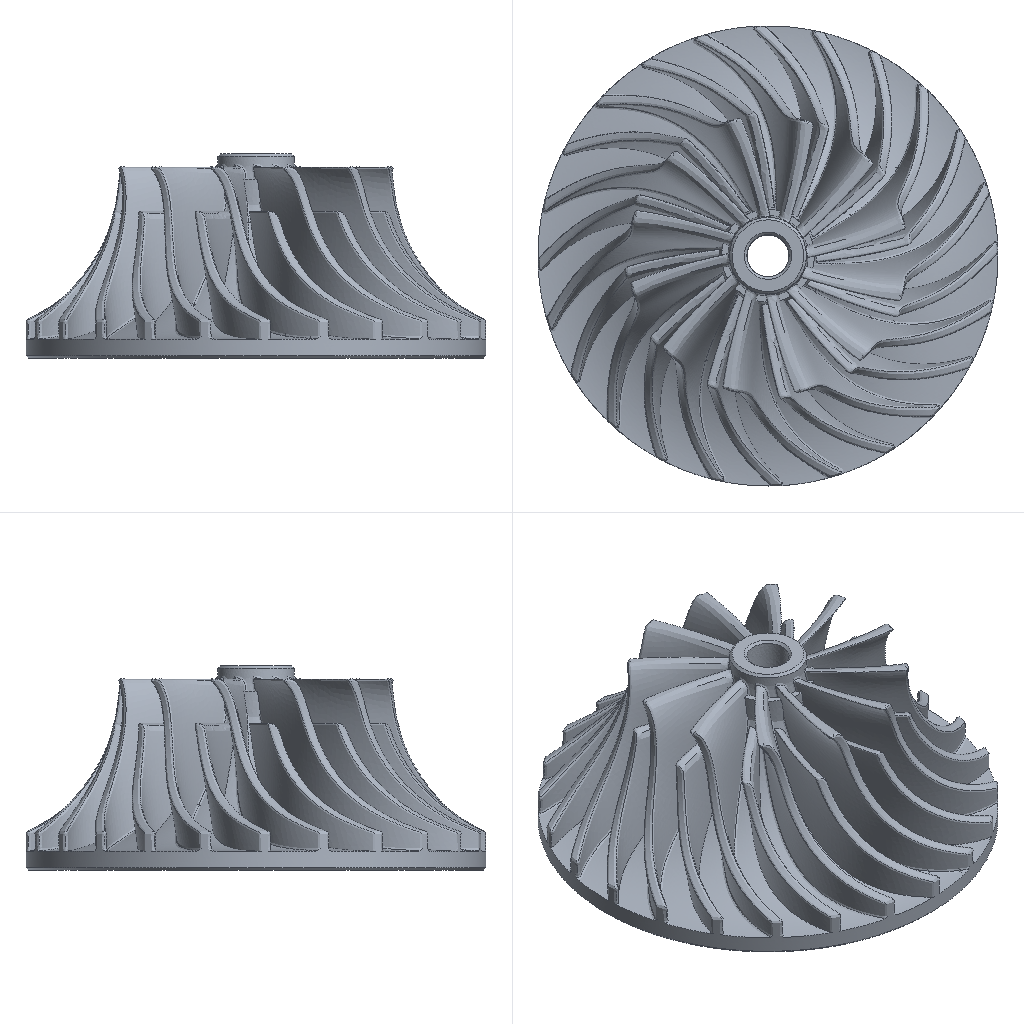Simulation study
Set-up summary:
category,name,step,type,value,unit,region
solver,ansys_mapdl
solver,version,,,22.2
units,MPA,,stated
analysis,deck,,static,static
load_step,requested,,,1
analysis,nlgeom,,,False
mesh,nodes,,,702794
mesh,elements,,,409743
element_type,ANSYS 187 (type 1),,solid,409743
load,load commands in deck,,count,1
bc,support commands in deck,,count,3
named_set,_DISPZEROUX,,component
named_set,_DISPZEROUY,,component
named_set,_DISPZEROUZ,,component
material,1,,in results
check,setup vs results,,match
Ansys APDL input file, long lists of numbers shortened:
/batch
/config,noeldb,1     ! force off writing results to database
*get,_wallstrt,active,,time,wall
! ANSYS input file written by Workbench version 2022 R2
! File used for geometry attach: D:\虚拟C盘\有限元\Impeller_v2.stp
/title,wbnew--____ (A5)
! ****** Begin Custom Load Command Snippet ******
/COM, ACT Extensions:
/COM,     LSDYNA, 2022.2
/COM,/COM,     ANSYSMotion, 2022.2
/COM,
! ****** End   Custom Load Command Snippet ******
*DIM,_wb_ProjectScratch_dir,string,248
_wb_ProjectScratch_dir(1) = 'C:\Users\16969\AppData\Local\Temp\WB_16969_1848_2\_ProjectScratch\ScrAECD\'
*DIM,_wb_SolverFiles_dir,string,248
_wb_SolverFiles_dir(1) = 'C:\Users\16969\AppData\Local\Temp\WB_16969_1848_2\wbnew_files\dp0\SYS\MECH\'
*DIM,_wb_userfiles_dir,string,248
_wb_userfiles_dir(1) = 'C:\Users\16969\AppData\Local\Temp\WB_16969_1848_2\wbnew_files\user_files\'
/com,--- Data in consistent NMM units. See Solving Units in the help system for more information.
/units,MPA
/nopr
/wb,file,start              !  signify a WB generated input file
/prep7
! Turn off shape checking because checks already performed inside WB mesher.
! See help system for more information.
SHPP,OFF,,NOWARN
/nolist
etcon,set             ! allow ANSYS to choose best KEYOP's for 180x elements, resets any applicable keyopt to MAPDL defaults
/com,*********** Nodes for the whole assembly ***********
nblock,3,,773073
(1i9,3e20.9e3)
        1    -1.739180704E+02     4.639509446E+01     1.500000000E+01
! (702793 more lines like these left out)
-1
/wb,elem,start            !  set before creation of elements
/com,*********** Elements for Body 1 "Impeller_v2-FreeParts|Impeller_v2" ***********
et,1,187
eblock,19,solid,,409743
(19i9)
        1        1        1        1        0        0        0        0       10        0        1    78715   108325    93396   101043   578094   670925   578088   578092
! (819485 more lines like these left out)
-1
/wb,elem,end               !  done creating elements
/com,*********** Send User Defined Coordinate System(s) ***********
csys,0
toffst,273.15,  ! Temperature offset from absolute zero
/com,*********** Set Reference Temperature ***********
tref,22.
/wb,mat,start              !  starting to send materials
/com,*********** Send Materials ***********
Temperature = 'TEMP' ! Temperature
MP,DENS,1,2.77e-09,	! tonne mm^-3
MP,ALPX,1,2.3e-05,	! C^-1
MP,C,1,875000000,	! mm^2 s^-2 C^-1
MPTEMP,,,,,,,,
MPTEMP,1,-100
MPTEMP,2,0
MPTEMP,3,100
MPTEMP,4,200
MPDATA,KXX,1, ,114,144,165,175,	! tonne mm s^-3 C^-1
MPTEMP,,,,,,,,
MPTEMP,,,,,,,,
MPTEMP,1,0
MPTEMP,2,20
MPTEMP,3,100
MPDATA,RSVX,1, ,2.43e-05,2.67e-05,3.63e-05,	! ohm mm
MPTEMP,,,,,,,,
MP,EX,1,75000,	! tonne s^-2 mm^-1
MP,NUXY,1,0.25,
MP,MURX,1,1,
/wb,mat,end                !  done sending materials
!************************* Model Summary ********************
!Impeller_v2-FreeParts|Impeller_v2,	铝合金,	matid,	1
!************************* End Model Summary ********************
! get the diagonal of the bounding box. Needed later for other things
*get,_xmin,node,,mnloc,x
*get,_ymin,node,,mnloc,y
*get,_zmin,node,,mnloc,z
*get,_xmax,node,,mxloc,x
*get,_ymax,node,,mxloc,y
*get,_zmax,node,,mxloc,z
_ASMDIAG=(_xmax-_xmin)*(_xmax-_xmin)+(_ymax-_ymin)*(_ymax-_ymin)+(_zmax-_zmin)*(_zmax-_zmin)
_ASMDIAG=SQRT(_ASMDIAG)
/wb,contact,start          !  starting to send contact
/wb,contact,end            !  done creating contacts
/golist
/wb,load,start             !  starting to send loads
/com,******* Constant Zero Displacement X *******
CMBLOCK,_DISPZEROUX,NODE,    11096
(8i10)
     19529     19530     19531     19532     19533     19534     19535     19536
! (1386 more lines like these left out)
cmsel,s,_DISPZEROUX
d,all,ux,0
nsel,all
/com,******* Constant Zero Displacement Y *******
CMBLOCK,_DISPZEROUY,NODE,    11096
(8i10)
     19529     19530     19531     19532     19533     19534     19535     19536
! (1386 more lines like these left out)
cmsel,s,_DISPZEROUY
d,all,uy,0
nsel,all
/com,******* Constant Zero Displacement Z *******
CMBLOCK,_DISPZEROUZ,NODE,    11096
(8i10)
     19529     19530     19531     19532     19533     19534     19535     19536
! (1386 more lines like these left out)
cmsel,s,_DISPZEROUZ
d,all,uz,0
nsel,all
/com,*********** Define Rotational Velocity ***********
cglo,0.,0.,80.
/gst,on,on
fini
*get,_numnode,node,0,count
*get,_numelem,elem,0,count
*get, _MAXELEMNUM, elem, 0, NUM, MAX
*get, _MAXNODENUM, node, 0, NUM, MAX
*get, _MAXELEMTYPE, etyp, 0, NUM, MAX
*get, _MAXREALCONST, rcon, 0, NUM, MAX
/go
/wb,load,end               !  done creating loads
/com,--- Number of total nodes = %_numnode%
/com,--- Number of contact elements = 0
/com,--- Number of spring elements = 0
/com,--- Number of bearing elements = 0
/com,--- Number of solid elements = 409743
/com,--- Number of condensed parts = 0
/com,--- Number of total elements = %_numelem%
*get,_wallbsol,active,,time,wall
/com,****************************************************************************
/com,*************************    SOLUTION       ********************************
/com,****************************************************************************
/solu
antype,0                   ! static analysis
_thickRatio=  1     ! Ratio of thick parts in the model
eqsl,pcg,1e-8,,,,,,1
cntr,print,1               ! print out contact info and also make no initial contact an error
dmpoption,emat,no             ! Don't combine emat file for DANSYS
dmpoption,esav,no             ! Don't combine esav file for DANSYS
nldiag,cont,iter           ! print out contact info each equilibrium iteration
rescontrol,,none                 ! Do not keep any restart files
/com,****************************************************
/com,******************* SOLVE FOR LS 1 OF 1 ****************
cgom,0.,0.,200.
/nopr
/gopr
nsub,1,1,1
time,1.
outres,erase
outres,all,none
outres,nsol,all,
outres,rsol,all
outres,eangl,all
outres,etmp,all
outres,veng,all
outres,strs,all,
outres,epel,all,
outres,eppl,all,
outres,cont,all,
! *********** WB SOLVE COMMAND ***********
! check interactive state
*get,ANSINTER_,active,,int
*if,ANSINTER_,ne,0,then
/eof
*endif
solve
/com *************** Write FE CONNECTORS *********
CEWRITE,file,ce,,INTE
/com,****************************************************
/com,*************** FINISHED SOLVE FOR LS 1 *************
*get,_wallasol,active,,time,wall
/nopr
*get,_numnode,node,0,count
*get,_numelem,elem,0,count
*get, _MAXELEMNUM, elem, 0, NUM, MAX
*get, _MAXNODENUM, node, 0, NUM, MAX,,,INTERNAL
*get, _MAXELEMTYPE, etyp, 0, NUM, MAX
*get, _MAXREALCONST, rcon, 0, NUM, MAX
*get,_NSOLTHREADS,active,0,ntfs
*get,_NSOLPROCESSES,active,0,npfs
/gopr
*get,_PCGITER,active,,solu,cgiter
/post1
xmlo,ENCODING,ISO-8859-1
xmlo,parm
/xml,parm,xml
fini
/gopr
*get,_walldone,active,,time,wall
_preptime=(_wallbsol-_wallstrt)*3600
_solvtime=(_wallasol-_wallbsol)*3600
_posttime=(_walldone-_wallasol)*3600
_totaltim=(_walldone-_wallstrt)*3600
*get,_dlbratio,active,0,solu,dlbr
*get,_combtime,active,0,solu,comb
*get,_ssmode,active,0,solu,ssmm
*get,_ndofs,active,0,solu,ndof
*get,_sol_end_time,active,0,set,time
*if,_sol_end_time,eq,1.,then
/fclean				!clean distributed files
*endif
/com,--- Total number of nodes = %_numnode%
/com,--- Total number of elements = %_numelem%
/com,--- Element load balance ratio = %_dlbratio%
/com,--- Time to combine distributed files = %_combtime%
/com,--- Sparse memory mode = %_ssmode%
/com,--- Number of DOF = %_ndofs%
/wb,file,end               ! done with WB generated input
Results summary:
result,analysis,,,static
result,last_loadstep,,,1
result,primary field,,,displacement
result,reaction total,1,FX,0.000797,N
result,reaction total,1,FY,0.003101,N
result,reaction total,1,FZ,2e-06,N
result,mass,,,0.009269,"NMM: mm, ton, N, s, mV, mA, degC"